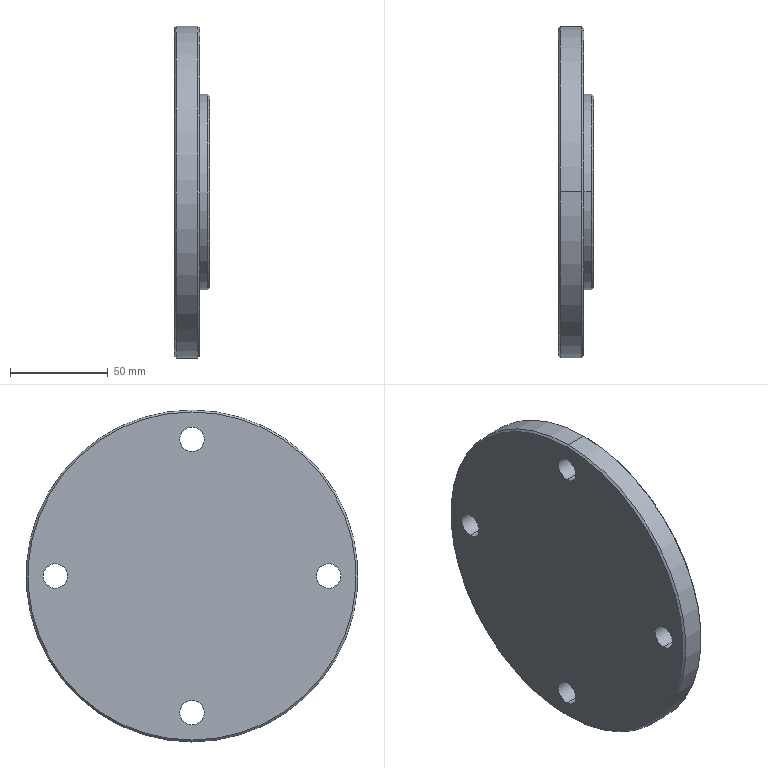Part | SolidWorks | features Chamfer 1, CirPattern 1, ICE 1, Revolution 1 | 1 solid | 26 faces | box 18 x 170 x 170 mm | volume 307921 mm3 | cylinder 14 | cone 8 | plane 4 | commonest cylinder face diameters 12.5 x8 70 x2 100 x2 170 x2
STEP:
#1=CARTESIAN_POINT('',(13.,0.,-84.));
#2=VERTEX_POINT('',#1);
#3=CARTESIAN_POINT('',(13.,0.,84.));
#4=VERTEX_POINT('',#3);
#5=CARTESIAN_POINT('',(13.,0.,0.));
#6=DIRECTION('',(1.,0.,0.));
#7=DIRECTION('',(0.,0.,1.));
#8=AXIS2_PLACEMENT_3D('',#5,#6,#7);
#9=CIRCLE('',#8,84.);
#10=EDGE_CURVE('',#2,#4,#9,.T.);
#11=ORIENTED_EDGE('',*,*,#10,.F.);
#12=CARTESIAN_POINT('',(12.,0.,-85.));
#13=VERTEX_POINT('',#12);
#14=CARTESIAN_POINT('',(12.,0.,-85.));
#15=DIRECTION('',(-0.7071,0.,-0.7071));
#16=VECTOR('',#15,1000.);
#17=LINE('',#14,#16);
#18=EDGE_CURVE('',#2,#13,#17,.T.);
#19=ORIENTED_EDGE('',*,*,#18,.T.);
#20=CARTESIAN_POINT('',(12.,0.,85.));
#21=VERTEX_POINT('',#20);
#22=CARTESIAN_POINT('',(12.,0.,0.));
#23=DIRECTION('',(-1.,0.,0.));
#24=DIRECTION('',(0.,0.,1.));
#25=AXIS2_PLACEMENT_3D('',#22,#23,#24);
#26=CIRCLE('',#25,85.);
#27=EDGE_CURVE('',#21,#13,#26,.T.);
#28=ORIENTED_EDGE('',*,*,#27,.F.);
#29=CARTESIAN_POINT('',(12.,0.,85.));
#30=DIRECTION('',(-0.7071,0.,0.7071));
#31=VECTOR('',#30,1000.);
#32=LINE('',#29,#31);
#33=EDGE_CURVE('',#4,#21,#32,.T.);
#34=ORIENTED_EDGE('',*,*,#33,.F.);
#35=EDGE_LOOP('',(#11,#19,#28,#34));
#36=FACE_OUTER_BOUND('',#35,.T.);
#37=CARTESIAN_POINT('',(12.,0.,0.));
#38=DIRECTION('',(-1.,0.,0.));
#39=DIRECTION('',(0.,0.,1.));
#40=AXIS2_PLACEMENT_3D('',#37,#38,#39);
#41=CONICAL_SURFACE('',#40,85.,0.7854);
#42=ADVANCED_FACE('',(#36),#41,.T.);
#43=CARTESIAN_POINT('',(0.,0.,84.));
#44=VERTEX_POINT('',#43);
#45=CARTESIAN_POINT('',(0.,0.,-84.));
#46=VERTEX_POINT('',#45);
#47=CARTESIAN_POINT('',(0.,0.,0.));
#48=DIRECTION('',(-1.,0.,0.));
#49=DIRECTION('',(0.,0.,-1.));
#50=AXIS2_PLACEMENT_3D('',#47,#48,#49);
#51=CIRCLE('',#50,84.);
#52=EDGE_CURVE('',#44,#46,#51,.T.);
#53=ORIENTED_EDGE('',*,*,#52,.F.);
#54=CARTESIAN_POINT('',(1.,0.,85.));
#55=VERTEX_POINT('',#54);
#56=CARTESIAN_POINT('',(0.,0.,84.));
#57=DIRECTION('',(0.7071,0.,0.7071));
#58=VECTOR('',#57,1000.);
#59=LINE('',#56,#58);
#60=EDGE_CURVE('',#44,#55,#59,.T.);
#61=ORIENTED_EDGE('',*,*,#60,.T.);
#62=CARTESIAN_POINT('',(1.,0.,-85.));
#63=VERTEX_POINT('',#62);
#64=CARTESIAN_POINT('',(1.,0.,0.));
#65=DIRECTION('',(1.,0.,0.));
#66=DIRECTION('',(0.,0.,-1.));
#67=AXIS2_PLACEMENT_3D('',#64,#65,#66);
#68=CIRCLE('',#67,85.);
#69=EDGE_CURVE('',#63,#55,#68,.T.);
#70=ORIENTED_EDGE('',*,*,#69,.F.);
#71=CARTESIAN_POINT('',(0.,0.,-84.));
#72=DIRECTION('',(0.7071,0.,-0.7071));
#73=VECTOR('',#72,1000.);
#74=LINE('',#71,#73);
#75=EDGE_CURVE('',#46,#63,#74,.T.);
#76=ORIENTED_EDGE('',*,*,#75,.F.);
#77=EDGE_LOOP('',(#53,#61,#70,#76));
#78=FACE_OUTER_BOUND('',#77,.T.);
#79=CARTESIAN_POINT('',(0.,0.,0.));
#80=DIRECTION('',(1.,0.,0.));
#81=DIRECTION('',(0.,0.,-1.));
#82=AXIS2_PLACEMENT_3D('',#79,#80,#81);
#83=CONICAL_SURFACE('',#82,84.,0.7854);
#84=ADVANCED_FACE('',(#78),#83,.T.);
#85=CARTESIAN_POINT('',(18.,0.,-49.));
#86=VERTEX_POINT('',#85);
#87=CARTESIAN_POINT('',(18.,0.,49.));
#88=VERTEX_POINT('',#87);
#89=CARTESIAN_POINT('',(18.,0.,0.));
#90=DIRECTION('',(1.,0.,0.));
#91=DIRECTION('',(0.,0.,1.));
#92=AXIS2_PLACEMENT_3D('',#89,#90,#91);
#93=CIRCLE('',#92,49.);
#94=EDGE_CURVE('',#86,#88,#93,.T.);
#95=ORIENTED_EDGE('',*,*,#94,.F.);
#96=CARTESIAN_POINT('',(17.,0.,-50.));
#97=VERTEX_POINT('',#96);
#98=CARTESIAN_POINT('',(17.,0.,-50.));
#99=DIRECTION('',(-0.7071,0.,-0.7071));
#100=VECTOR('',#99,1000.);
#101=LINE('',#98,#100);
#102=EDGE_CURVE('',#86,#97,#101,.T.);
#103=ORIENTED_EDGE('',*,*,#102,.T.);
#104=CARTESIAN_POINT('',(17.,0.,50.));
#105=VERTEX_POINT('',#104);
#106=CARTESIAN_POINT('',(17.,0.,0.));
#107=DIRECTION('',(-1.,0.,0.));
#108=DIRECTION('',(0.,0.,1.));
#109=AXIS2_PLACEMENT_3D('',#106,#107,#108);
#110=CIRCLE('',#109,50.);
#111=EDGE_CURVE('',#105,#97,#110,.T.);
#112=ORIENTED_EDGE('',*,*,#111,.F.);
#113=CARTESIAN_POINT('',(17.,0.,50.));
#114=DIRECTION('',(-0.7071,0.,0.7071));
#115=VECTOR('',#114,1000.);
#116=LINE('',#113,#115);
#117=EDGE_CURVE('',#88,#105,#116,.T.);
#118=ORIENTED_EDGE('',*,*,#117,.F.);
#119=EDGE_LOOP('',(#95,#103,#112,#118));
#120=FACE_OUTER_BOUND('',#119,.T.);
#121=CARTESIAN_POINT('',(17.,0.,0.));
#122=DIRECTION('',(-1.,0.,0.));
#123=DIRECTION('',(0.,0.,1.));
#124=AXIS2_PLACEMENT_3D('',#121,#122,#123);
#125=CONICAL_SURFACE('',#124,50.,0.7854);
#126=ADVANCED_FACE('',(#120),#125,.T.);
#127=CARTESIAN_POINT('',(17.,0.,35.));
#128=VERTEX_POINT('',#127);
#129=CARTESIAN_POINT('',(17.,0.,-35.));
#130=VERTEX_POINT('',#129);
#131=CARTESIAN_POINT('',(17.,0.,0.));
#132=DIRECTION('',(1.,0.,0.));
#133=DIRECTION('',(0.,0.,1.));
#134=AXIS2_PLACEMENT_3D('',#131,#132,#133);
#135=CIRCLE('',#134,35.);
#136=EDGE_CURVE('',#128,#130,#135,.T.);
#137=ORIENTED_EDGE('',*,*,#136,.F.);
#138=CARTESIAN_POINT('',(18.,0.,36.));
#139=VERTEX_POINT('',#138);
#140=CARTESIAN_POINT('',(18.,0.,36.));
#141=DIRECTION('',(0.7071,0.,0.7071));
#142=VECTOR('',#141,1000.);
#143=LINE('',#140,#142);
#144=EDGE_CURVE('',#128,#139,#143,.T.);
#145=ORIENTED_EDGE('',*,*,#144,.T.);
#146=CARTESIAN_POINT('',(18.,0.,-36.));
#147=VERTEX_POINT('',#146);
#148=CARTESIAN_POINT('',(18.,0.,0.));
#149=DIRECTION('',(-1.,0.,0.));
#150=DIRECTION('',(0.,0.,1.));
#151=AXIS2_PLACEMENT_3D('',#148,#149,#150);
#152=CIRCLE('',#151,36.);
#153=EDGE_CURVE('',#147,#139,#152,.T.);
#154=ORIENTED_EDGE('',*,*,#153,.F.);
#155=CARTESIAN_POINT('',(18.,0.,-36.));
#156=DIRECTION('',(0.7071,0.,-0.7071));
#157=VECTOR('',#156,1000.);
#158=LINE('',#155,#157);
#159=EDGE_CURVE('',#130,#147,#158,.T.);
#160=ORIENTED_EDGE('',*,*,#159,.F.);
#161=EDGE_LOOP('',(#137,#145,#154,#160));
#162=FACE_OUTER_BOUND('',#161,.T.);
#163=CARTESIAN_POINT('',(18.,0.,0.));
#164=DIRECTION('',(1.,0.,0.));
#165=DIRECTION('',(0.,0.,-1.));
#166=AXIS2_PLACEMENT_3D('',#163,#164,#165);
#167=CONICAL_SURFACE('',#166,36.,0.7854);
#168=ADVANCED_FACE('',(#162),#167,.F.);
#169=CARTESIAN_POINT('',(13.,-70.,-6.25));
#170=VERTEX_POINT('',#169);
#171=CARTESIAN_POINT('',(13.,-70.,6.25));
#172=VERTEX_POINT('',#171);
#173=CARTESIAN_POINT('',(13.,-70.,0.));
#174=DIRECTION('',(-1.,0.,0.));
#175=DIRECTION('',(0.,0.,1.));
#176=AXIS2_PLACEMENT_3D('',#173,#174,#175);
#177=CIRCLE('',#176,6.25);
#178=EDGE_CURVE('',#170,#172,#177,.T.);
#179=ORIENTED_EDGE('',*,*,#178,.F.);
#180=CARTESIAN_POINT('',(0.,-70.,-6.25));
#181=VERTEX_POINT('',#180);
#182=CARTESIAN_POINT('',(18.,-70.,-6.25));
#183=DIRECTION('',(-1.,0.,0.));
#184=VECTOR('',#183,1000.);
#185=LINE('',#182,#184);
#186=EDGE_CURVE('',#170,#181,#185,.T.);
#187=ORIENTED_EDGE('',*,*,#186,.T.);
#188=CARTESIAN_POINT('',(0.,-70.,6.25));
#189=VERTEX_POINT('',#188);
#190=CARTESIAN_POINT('',(0.,-70.,0.));
#191=DIRECTION('',(-1.,0.,0.));
#192=DIRECTION('',(0.,0.,-1.));
#193=AXIS2_PLACEMENT_3D('',#190,#191,#192);
#194=CIRCLE('',#193,6.25);
#195=EDGE_CURVE('',#181,#189,#194,.T.);
#196=ORIENTED_EDGE('',*,*,#195,.T.);
#197=CARTESIAN_POINT('',(18.,-70.,6.25));
#198=DIRECTION('',(-1.,0.,0.));
#199=VECTOR('',#198,1000.);
#200=LINE('',#197,#199);
#201=EDGE_CURVE('',#172,#189,#200,.T.);
#202=ORIENTED_EDGE('',*,*,#201,.F.);
#203=EDGE_LOOP('',(#179,#187,#196,#202));
#204=FACE_OUTER_BOUND('',#203,.T.);
#205=CARTESIAN_POINT('',(18.,-70.,0.));
#206=DIRECTION('',(-1.,0.,0.));
#207=DIRECTION('',(0.,0.,1.));
#208=AXIS2_PLACEMENT_3D('',#205,#206,#207);
#209=CYLINDRICAL_SURFACE('',#208,6.25);
#210=ADVANCED_FACE('',(#204),#209,.F.);
#211=CARTESIAN_POINT('',(13.,0.,63.75));
#212=VERTEX_POINT('',#211);
#213=CARTESIAN_POINT('',(13.,0.,76.25));
#214=VERTEX_POINT('',#213);
#215=CARTESIAN_POINT('',(13.,0.,70.));
#216=DIRECTION('',(-1.,0.,0.));
#217=DIRECTION('',(0.,0.,1.));
#218=AXIS2_PLACEMENT_3D('',#215,#216,#217);
#219=CIRCLE('',#218,6.25);
#220=EDGE_CURVE('',#212,#214,#219,.T.);
#221=ORIENTED_EDGE('',*,*,#220,.F.);
#222=CARTESIAN_POINT('',(0.,0.,63.75));
#223=VERTEX_POINT('',#222);
#224=CARTESIAN_POINT('',(18.,0.,63.75));
#225=DIRECTION('',(-1.,0.,0.));
#226=VECTOR('',#225,1000.);
#227=LINE('',#224,#226);
#228=EDGE_CURVE('',#212,#223,#227,.T.);
#229=ORIENTED_EDGE('',*,*,#228,.T.);
#230=CARTESIAN_POINT('',(0.,0.,76.25));
#231=VERTEX_POINT('',#230);
#232=CARTESIAN_POINT('',(0.,0.,70.));
#233=DIRECTION('',(-1.,0.,0.));
#234=DIRECTION('',(0.,-1.,0.));
#235=AXIS2_PLACEMENT_3D('',#232,#233,#234);
#236=CIRCLE('',#235,6.25);
#237=EDGE_CURVE('',#223,#231,#236,.T.);
#238=ORIENTED_EDGE('',*,*,#237,.T.);
#239=CARTESIAN_POINT('',(18.,0.,76.25));
#240=DIRECTION('',(-1.,0.,0.));
#241=VECTOR('',#240,1000.);
#242=LINE('',#239,#241);
#243=EDGE_CURVE('',#214,#231,#242,.T.);
#244=ORIENTED_EDGE('',*,*,#243,.F.);
#245=EDGE_LOOP('',(#221,#229,#238,#244));
#246=FACE_OUTER_BOUND('',#245,.T.);
#247=CARTESIAN_POINT('',(18.,0.,70.));
#248=DIRECTION('',(-1.,0.,0.));
#249=DIRECTION('',(0.,0.,1.));
#250=AXIS2_PLACEMENT_3D('',#247,#248,#249);
#251=CYLINDRICAL_SURFACE('',#250,6.25);
#252=ADVANCED_FACE('',(#246),#251,.F.);
#253=CARTESIAN_POINT('',(13.,0.,-76.25));
#254=VERTEX_POINT('',#253);
#255=CARTESIAN_POINT('',(13.,0.,-63.75));
#256=VERTEX_POINT('',#255);
#257=CARTESIAN_POINT('',(13.,0.,-70.));
#258=DIRECTION('',(-1.,0.,0.));
#259=DIRECTION('',(0.,0.,1.));
#260=AXIS2_PLACEMENT_3D('',#257,#258,#259);
#261=CIRCLE('',#260,6.25);
#262=EDGE_CURVE('',#254,#256,#261,.T.);
#263=ORIENTED_EDGE('',*,*,#262,.F.);
#264=CARTESIAN_POINT('',(0.,0.,-76.25));
#265=VERTEX_POINT('',#264);
#266=CARTESIAN_POINT('',(18.,0.,-76.25));
#267=DIRECTION('',(-1.,0.,0.));
#268=VECTOR('',#267,1000.);
#269=LINE('',#266,#268);
#270=EDGE_CURVE('',#254,#265,#269,.T.);
#271=ORIENTED_EDGE('',*,*,#270,.T.);
#272=CARTESIAN_POINT('',(0.,0.,-63.75));
#273=VERTEX_POINT('',#272);
#274=CARTESIAN_POINT('',(0.,0.,-70.));
#275=DIRECTION('',(-1.,0.,0.));
#276=DIRECTION('',(0.,1.,0.));
#277=AXIS2_PLACEMENT_3D('',#274,#275,#276);
#278=CIRCLE('',#277,6.25);
#279=EDGE_CURVE('',#265,#273,#278,.T.);
#280=ORIENTED_EDGE('',*,*,#279,.T.);
#281=CARTESIAN_POINT('',(18.,0.,-63.75));
#282=DIRECTION('',(-1.,0.,0.));
#283=VECTOR('',#282,1000.);
#284=LINE('',#281,#283);
#285=EDGE_CURVE('',#256,#273,#284,.T.);
#286=ORIENTED_EDGE('',*,*,#285,.F.);
#287=EDGE_LOOP('',(#263,#271,#280,#286));
#288=FACE_OUTER_BOUND('',#287,.T.);
#289=CARTESIAN_POINT('',(18.,0.,-70.));
#290=DIRECTION('',(-1.,0.,0.));
#291=DIRECTION('',(0.,0.,1.));
#292=AXIS2_PLACEMENT_3D('',#289,#290,#291);
#293=CYLINDRICAL_SURFACE('',#292,6.25);
#294=ADVANCED_FACE('',(#288),#293,.F.);
#295=CARTESIAN_POINT('',(13.,70.,-6.25));
#296=VERTEX_POINT('',#295);
#297=CARTESIAN_POINT('',(13.,70.,6.25));
#298=VERTEX_POINT('',#297);
#299=CARTESIAN_POINT('',(13.,70.,0.));
#300=DIRECTION('',(-1.,0.,0.));
#301=DIRECTION('',(0.,0.,1.));
#302=AXIS2_PLACEMENT_3D('',#299,#300,#301);
#303=CIRCLE('',#302,6.25);
#304=EDGE_CURVE('',#296,#298,#303,.T.);
#305=ORIENTED_EDGE('',*,*,#304,.F.);
#306=CARTESIAN_POINT('',(0.,70.,-6.25));
#307=VERTEX_POINT('',#306);
#308=CARTESIAN_POINT('',(18.,70.,-6.25));
#309=DIRECTION('',(-1.,0.,0.));
#310=VECTOR('',#309,1000.);
#311=LINE('',#308,#310);
#312=EDGE_CURVE('',#296,#307,#311,.T.);
#313=ORIENTED_EDGE('',*,*,#312,.T.);
#314=CARTESIAN_POINT('',(0.,70.,6.25));
#315=VERTEX_POINT('',#314);
#316=CARTESIAN_POINT('',(0.,70.,0.));
#317=DIRECTION('',(-1.,0.,0.));
#318=DIRECTION('',(0.,0.,1.));
#319=AXIS2_PLACEMENT_3D('',#316,#317,#318);
#320=CIRCLE('',#319,6.25);
#321=EDGE_CURVE('',#307,#315,#320,.T.);
#322=ORIENTED_EDGE('',*,*,#321,.T.);
#323=CARTESIAN_POINT('',(18.,70.,6.25));
#324=DIRECTION('',(-1.,0.,0.));
#325=VECTOR('',#324,1000.);
#326=LINE('',#323,#325);
#327=EDGE_CURVE('',#298,#315,#326,.T.);
#328=ORIENTED_EDGE('',*,*,#327,.F.);
#329=EDGE_LOOP('',(#305,#313,#322,#328));
#330=FACE_OUTER_BOUND('',#329,.T.);
#331=CARTESIAN_POINT('',(18.,70.,0.));
#332=DIRECTION('',(-1.,0.,0.));
#333=DIRECTION('',(0.,0.,1.));
#334=AXIS2_PLACEMENT_3D('',#331,#332,#333);
#335=CYLINDRICAL_SURFACE('',#334,6.25);
#336=ADVANCED_FACE('',(#330),#335,.F.);
#337=ORIENTED_EDGE('',*,*,#136,.T.);
#338=CARTESIAN_POINT('',(13.,0.,-35.));
#339=VERTEX_POINT('',#338);
#340=CARTESIAN_POINT('',(0.,0.,-35.));
#341=DIRECTION('',(-1.,0.,0.));
#342=VECTOR('',#341,1000.);
#343=LINE('',#340,#342);
#344=EDGE_CURVE('',#130,#339,#343,.T.);
#345=ORIENTED_EDGE('',*,*,#344,.T.);
#346=CARTESIAN_POINT('',(13.,0.,35.));
#347=VERTEX_POINT('',#346);
#348=CARTESIAN_POINT('',(13.,0.,0.));
#349=DIRECTION('',(-1.,0.,0.));
#350=DIRECTION('',(0.,0.,1.));
#351=AXIS2_PLACEMENT_3D('',#348,#349,#350);
#352=CIRCLE('',#351,35.);
#353=EDGE_CURVE('',#339,#347,#352,.T.);
#354=ORIENTED_EDGE('',*,*,#353,.T.);
#355=CARTESIAN_POINT('',(0.,0.,35.));
#356=DIRECTION('',(-1.,0.,0.));
#357=VECTOR('',#356,1000.);
#358=LINE('',#355,#357);
#359=EDGE_CURVE('',#128,#347,#358,.T.);
#360=ORIENTED_EDGE('',*,*,#359,.F.);
#361=EDGE_LOOP('',(#337,#345,#354,#360));
#362=FACE_OUTER_BOUND('',#361,.T.);
#363=CARTESIAN_POINT('',(0.,0.,0.));
#364=DIRECTION('',(-1.,0.,0.));
#365=DIRECTION('',(0.,0.,1.));
#366=AXIS2_PLACEMENT_3D('',#363,#364,#365);
#367=CYLINDRICAL_SURFACE('',#366,35.);
#368=ADVANCED_FACE('',(#362),#367,.F.);
#369=ORIENTED_EDGE('',*,*,#111,.T.);
#370=CARTESIAN_POINT('',(13.,0.,-50.));
#371=VERTEX_POINT('',#370);
#372=CARTESIAN_POINT('',(0.,0.,-50.));
#373=DIRECTION('',(-1.,0.,0.));
#374=VECTOR('',#373,1000.);
#375=LINE('',#372,#374);
#376=EDGE_CURVE('',#97,#371,#375,.T.);
#377=ORIENTED_EDGE('',*,*,#376,.T.);
#378=CARTESIAN_POINT('',(13.,0.,50.));
#379=VERTEX_POINT('',#378);
#380=CARTESIAN_POINT('',(13.,0.,0.));
#381=DIRECTION('',(-1.,0.,0.));
#382=DIRECTION('',(0.,0.,1.));
#383=AXIS2_PLACEMENT_3D('',#380,#381,#382);
#384=CIRCLE('',#383,50.);
#385=EDGE_CURVE('',#379,#371,#384,.T.);
#386=ORIENTED_EDGE('',*,*,#385,.F.);
#387=CARTESIAN_POINT('',(0.,0.,50.));
#388=DIRECTION('',(-1.,0.,0.));
#389=VECTOR('',#388,1000.);
#390=LINE('',#387,#389);
#391=EDGE_CURVE('',#105,#379,#390,.T.);
#392=ORIENTED_EDGE('',*,*,#391,.F.);
#393=EDGE_LOOP('',(#369,#377,#386,#392));
#394=FACE_OUTER_BOUND('',#393,.T.);
#395=CARTESIAN_POINT('',(0.,0.,0.));
#396=DIRECTION('',(-1.,0.,0.));
#397=DIRECTION('',(0.,0.,1.));
#398=AXIS2_PLACEMENT_3D('',#395,#396,#397);
#399=CYLINDRICAL_SURFACE('',#398,50.);
#400=ADVANCED_FACE('',(#394),#399,.T.);
#401=ORIENTED_EDGE('',*,*,#27,.T.);
#402=CARTESIAN_POINT('',(0.,0.,-85.));
#403=DIRECTION('',(-1.,0.,0.));
#404=VECTOR('',#403,1000.);
#405=LINE('',#402,#404);
#406=EDGE_CURVE('',#13,#63,#405,.T.);
#407=ORIENTED_EDGE('',*,*,#406,.T.);
#408=ORIENTED_EDGE('',*,*,#69,.T.);
#409=CARTESIAN_POINT('',(0.,0.,85.));
#410=DIRECTION('',(-1.,0.,0.));
#411=VECTOR('',#410,1000.);
#412=LINE('',#409,#411);
#413=EDGE_CURVE('',#21,#55,#412,.T.);
#414=ORIENTED_EDGE('',*,*,#413,.F.);
#415=EDGE_LOOP('',(#401,#407,#408,#414));
#416=FACE_OUTER_BOUND('',#415,.T.);
#417=CARTESIAN_POINT('',(0.,0.,0.));
#418=DIRECTION('',(-1.,0.,0.));
#419=DIRECTION('',(0.,0.,1.));
#420=AXIS2_PLACEMENT_3D('',#417,#418,#419);
#421=CYLINDRICAL_SURFACE('',#420,85.);
#422=ADVANCED_FACE('',(#416),#421,.T.);
#423=CARTESIAN_POINT('',(0.,0.,0.));
#424=DIRECTION('',(-1.,0.,0.));
#425=DIRECTION('',(0.,0.,-1.));
#426=AXIS2_PLACEMENT_3D('',#423,#424,#425);
#427=CIRCLE('',#426,84.);
#428=EDGE_CURVE('',#46,#44,#427,.T.);
#429=ORIENTED_EDGE('',*,*,#428,.T.);
#430=ORIENTED_EDGE('',*,*,#52,.T.);
#431=EDGE_LOOP('',(#429,#430));
#432=FACE_OUTER_BOUND('',#431,.T.);
#433=CARTESIAN_POINT('',(0.,-70.,0.));
#434=DIRECTION('',(-1.,0.,0.));
#435=DIRECTION('',(0.,0.,-1.));
#436=AXIS2_PLACEMENT_3D('',#433,#434,#435);
#437=CIRCLE('',#436,6.25);
#438=EDGE_CURVE('',#189,#181,#437,.T.);
#439=ORIENTED_EDGE('',*,*,#438,.F.);
#440=ORIENTED_EDGE('',*,*,#195,.F.);
#441=EDGE_LOOP('',(#439,#440));
#442=FACE_BOUND('',#441,.T.);
#443=CARTESIAN_POINT('',(0.,0.,70.));
#444=DIRECTION('',(-1.,0.,0.));
#445=DIRECTION('',(0.,-1.,0.));
#446=AXIS2_PLACEMENT_3D('',#443,#444,#445);
#447=CIRCLE('',#446,6.25);
#448=EDGE_CURVE('',#231,#223,#447,.T.);
#449=ORIENTED_EDGE('',*,*,#448,.F.);
#450=ORIENTED_EDGE('',*,*,#237,.F.);
#451=EDGE_LOOP('',(#449,#450));
#452=FACE_BOUND('',#451,.T.);
#453=CARTESIAN_POINT('',(0.,0.,-70.));
#454=DIRECTION('',(-1.,0.,0.));
#455=DIRECTION('',(0.,1.,0.));
#456=AXIS2_PLACEMENT_3D('',#453,#454,#455);
#457=CIRCLE('',#456,6.25);
#458=EDGE_CURVE('',#273,#265,#457,.T.);
#459=ORIENTED_EDGE('',*,*,#458,.F.);
#460=ORIENTED_EDGE('',*,*,#279,.F.);
#461=EDGE_LOOP('',(#459,#460));
#462=FACE_BOUND('',#461,.T.);
#463=CARTESIAN_POINT('',(0.,70.,0.));
#464=DIRECTION('',(-1.,0.,0.));
#465=DIRECTION('',(0.,0.,1.));
#466=AXIS2_PLACEMENT_3D('',#463,#464,#465);
#467=CIRCLE('',#466,6.25);
#468=EDGE_CURVE('',#315,#307,#467,.T.);
#469=ORIENTED_EDGE('',*,*,#468,.F.);
#470=ORIENTED_EDGE('',*,*,#321,.F.);
#471=EDGE_LOOP('',(#469,#470));
#472=FACE_BOUND('',#471,.T.);
#473=CARTESIAN_POINT('',(0.,0.,0.));
#474=DIRECTION('',(1.,0.,0.));
#475=DIRECTION('',(0.,0.,-1.));
#476=AXIS2_PLACEMENT_3D('',#473,#474,#475);
#477=PLANE('',#476);
#478=ADVANCED_FACE('',(#432,#442,#452,#462,#472),#477,.F.);
#479=ORIENTED_EDGE('',*,*,#406,.F.);
#480=CARTESIAN_POINT('',(12.,0.,0.));
#481=DIRECTION('',(-1.,0.,0.));
#482=DIRECTION('',(0.,0.,1.));
#483=AXIS2_PLACEMENT_3D('',#480,#481,#482);
#484=CIRCLE('',#483,85.);
#485=EDGE_CURVE('',#13,#21,#484,.T.);
#486=ORIENTED_EDGE('',*,*,#485,.T.);
#487=ORIENTED_EDGE('',*,*,#413,.T.);
#488=CARTESIAN_POINT('',(1.,0.,0.));
#489=DIRECTION('',(1.,0.,0.));
#490=DIRECTION('',(0.,0.,-1.));
#491=AXIS2_PLACEMENT_3D('',#488,#489,#490);
#492=CIRCLE('',#491,85.);
#493=EDGE_CURVE('',#55,#63,#492,.T.);
#494=ORIENTED_EDGE('',*,*,#493,.T.);
#495=EDGE_LOOP('',(#479,#486,#487,#494));
#496=FACE_OUTER_BOUND('',#495,.T.);
#497=CARTESIAN_POINT('',(0.,0.,0.));
#498=DIRECTION('',(-1.,0.,0.));
#499=DIRECTION('',(0.,0.,1.));
#500=AXIS2_PLACEMENT_3D('',#497,#498,#499);
#501=CYLINDRICAL_SURFACE('',#500,85.);
#502=ADVANCED_FACE('',(#496),#501,.T.);
#503=CARTESIAN_POINT('',(13.,0.,0.));
#504=DIRECTION('',(1.,0.,0.));
#505=DIRECTION('',(0.,0.,1.));
#506=AXIS2_PLACEMENT_3D('',#503,#504,#505);
#507=CIRCLE('',#506,84.);
#508=EDGE_CURVE('',#4,#2,#507,.T.);
#509=ORIENTED_EDGE('',*,*,#508,.T.);
#510=ORIENTED_EDGE('',*,*,#10,.T.);
#511=EDGE_LOOP('',(#509,#510));
#512=FACE_OUTER_BOUND('',#511,.T.);
#513=CARTESIAN_POINT('',(13.,-70.,0.));
#514=DIRECTION('',(-1.,0.,0.));
#515=DIRECTION('',(0.,0.,1.));
#516=AXIS2_PLACEMENT_3D('',#513,#514,#515);
#517=CIRCLE('',#516,6.25);
#518=EDGE_CURVE('',#172,#170,#517,.T.);
#519=ORIENTED_EDGE('',*,*,#518,.T.);
#520=ORIENTED_EDGE('',*,*,#178,.T.);
#521=EDGE_LOOP('',(#519,#520));
#522=FACE_BOUND('',#521,.T.);
#523=CARTESIAN_POINT('',(13.,0.,70.));
#524=DIRECTION('',(-1.,0.,0.));
#525=DIRECTION('',(0.,0.,1.));
#526=AXIS2_PLACEMENT_3D('',#523,#524,#525);
#527=CIRCLE('',#526,6.25);
#528=EDGE_CURVE('',#214,#212,#527,.T.);
#529=ORIENTED_EDGE('',*,*,#528,.T.);
#530=ORIENTED_EDGE('',*,*,#220,.T.);
#531=EDGE_LOOP('',(#529,#530));
#532=FACE_BOUND('',#531,.T.);
#533=CARTESIAN_POINT('',(13.,0.,-70.));
#534=DIRECTION('',(-1.,0.,0.));
#535=DIRECTION('',(0.,0.,1.));
#536=AXIS2_PLACEMENT_3D('',#533,#534,#535);
#537=CIRCLE('',#536,6.25);
#538=EDGE_CURVE('',#256,#254,#537,.T.);
#539=ORIENTED_EDGE('',*,*,#538,.T.);
#540=ORIENTED_EDGE('',*,*,#262,.T.);
#541=EDGE_LOOP('',(#539,#540));
#542=FACE_BOUND('',#541,.T.);
#543=CARTESIAN_POINT('',(13.,70.,0.));
#544=DIRECTION('',(-1.,0.,0.));
#545=DIRECTION('',(0.,0.,1.));
#546=AXIS2_PLACEMENT_3D('',#543,#544,#545);
#547=CIRCLE('',#546,6.25);
#548=EDGE_CURVE('',#298,#296,#547,.T.);
#549=ORIENTED_EDGE('',*,*,#548,.T.);
#550=ORIENTED_EDGE('',*,*,#304,.T.);
#551=EDGE_LOOP('',(#549,#550));
#552=FACE_BOUND('',#551,.T.);
#553=ORIENTED_EDGE('',*,*,#385,.T.);
#554=CARTESIAN_POINT('',(13.,0.,0.));
#555=DIRECTION('',(-1.,0.,0.));
#556=DIRECTION('',(0.,0.,1.));
#557=AXIS2_PLACEMENT_3D('',#554,#555,#556);
#558=CIRCLE('',#557,50.);
#559=EDGE_CURVE('',#371,#379,#558,.T.);
#560=ORIENTED_EDGE('',*,*,#559,.T.);
#561=EDGE_LOOP('',(#553,#560));
#562=FACE_BOUND('',#561,.T.);
#563=CARTESIAN_POINT('',(13.,85.,0.));
#564=DIRECTION('',(-1.,0.,0.));
#565=DIRECTION('',(0.,0.,1.));
#566=AXIS2_PLACEMENT_3D('',#563,#564,#565);
#567=PLANE('',#566);
#568=ADVANCED_FACE('',(#512,#522,#532,#542,#552,#562),#567,.F.);
#569=ORIENTED_EDGE('',*,*,#376,.F.);
#570=CARTESIAN_POINT('',(17.,0.,0.));
#571=DIRECTION('',(-1.,0.,0.));
#572=DIRECTION('',(0.,0.,1.));
#573=AXIS2_PLACEMENT_3D('',#570,#571,#572);
#574=CIRCLE('',#573,50.);
#575=EDGE_CURVE('',#97,#105,#574,.T.);
#576=ORIENTED_EDGE('',*,*,#575,.T.);
#577=ORIENTED_EDGE('',*,*,#391,.T.);
#578=ORIENTED_EDGE('',*,*,#559,.F.);
#579=EDGE_LOOP('',(#569,#576,#577,#578));
#580=FACE_OUTER_BOUND('',#579,.T.);
#581=CARTESIAN_POINT('',(0.,0.,0.));
#582=DIRECTION('',(-1.,0.,0.));
#583=DIRECTION('',(0.,0.,1.));
#584=AXIS2_PLACEMENT_3D('',#581,#582,#583);
#585=CYLINDRICAL_SURFACE('',#584,50.);
#586=ADVANCED_FACE('',(#580),#585,.T.);
#587=ORIENTED_EDGE('',*,*,#153,.T.);
#588=CARTESIAN_POINT('',(18.,0.,0.));
#589=DIRECTION('',(-1.,0.,0.));
#590=DIRECTION('',(0.,0.,1.));
#591=AXIS2_PLACEMENT_3D('',#588,#589,#590);
#592=CIRCLE('',#591,36.);
#593=EDGE_CURVE('',#139,#147,#592,.T.);
#594=ORIENTED_EDGE('',*,*,#593,.T.);
#595=EDGE_LOOP('',(#587,#594));
#596=FACE_BOUND('',#595,.T.);
#597=CARTESIAN_POINT('',(18.,0.,0.));
#598=DIRECTION('',(1.,0.,0.));
#599=DIRECTION('',(0.,0.,1.));
#600=AXIS2_PLACEMENT_3D('',#597,#598,#599);
#601=CIRCLE('',#600,49.);
#602=EDGE_CURVE('',#88,#86,#601,.T.);
#603=ORIENTED_EDGE('',*,*,#602,.T.);
#604=ORIENTED_EDGE('',*,*,#94,.T.);
#605=EDGE_LOOP('',(#603,#604));
#606=FACE_OUTER_BOUND('',#605,.T.);
#607=CARTESIAN_POINT('',(18.,50.,0.));
#608=DIRECTION('',(-1.,0.,0.));
#609=DIRECTION('',(0.,0.,1.));
#610=AXIS2_PLACEMENT_3D('',#607,#608,#609);
#611=PLANE('',#610);
#612=ADVANCED_FACE('',(#596,#606),#611,.F.);
#613=ORIENTED_EDGE('',*,*,#344,.F.);
#614=CARTESIAN_POINT('',(17.,0.,0.));
#615=DIRECTION('',(1.,0.,0.));
#616=DIRECTION('',(0.,0.,1.));
#617=AXIS2_PLACEMENT_3D('',#614,#615,#616);
#618=CIRCLE('',#617,35.);
#619=EDGE_CURVE('',#130,#128,#618,.T.);
#620=ORIENTED_EDGE('',*,*,#619,.T.);
#621=ORIENTED_EDGE('',*,*,#359,.T.);
#622=CARTESIAN_POINT('',(13.,0.,0.));
#623=DIRECTION('',(-1.,0.,0.));
#624=DIRECTION('',(0.,0.,1.));
#625=AXIS2_PLACEMENT_3D('',#622,#623,#624);
#626=CIRCLE('',#625,35.);
#627=EDGE_CURVE('',#347,#339,#626,.T.);
#628=ORIENTED_EDGE('',*,*,#627,.T.);
#629=EDGE_LOOP('',(#613,#620,#621,#628));
#630=FACE_OUTER_BOUND('',#629,.T.);
#631=CARTESIAN_POINT('',(0.,0.,0.));
#632=DIRECTION('',(-1.,0.,0.));
#633=DIRECTION('',(0.,0.,1.));
#634=AXIS2_PLACEMENT_3D('',#631,#632,#633);
#635=CYLINDRICAL_SURFACE('',#634,35.);
#636=ADVANCED_FACE('',(#630),#635,.F.);
#637=ORIENTED_EDGE('',*,*,#627,.F.);
#638=ORIENTED_EDGE('',*,*,#353,.F.);
#639=EDGE_LOOP('',(#637,#638));
#640=FACE_OUTER_BOUND('',#639,.T.);
#641=CARTESIAN_POINT('',(13.,35.,0.));
#642=DIRECTION('',(-1.,0.,0.));
#643=DIRECTION('',(0.,0.,1.));
#644=AXIS2_PLACEMENT_3D('',#641,#642,#643);
#645=PLANE('',#644);
#646=ADVANCED_FACE('',(#640),#645,.F.);
#647=ORIENTED_EDGE('',*,*,#312,.F.);
#648=ORIENTED_EDGE('',*,*,#548,.F.);
#649=ORIENTED_EDGE('',*,*,#327,.T.);
#650=ORIENTED_EDGE('',*,*,#468,.T.);
#651=EDGE_LOOP('',(#647,#648,#649,#650));
#652=FACE_OUTER_BOUND('',#651,.T.);
#653=CARTESIAN_POINT('',(18.,70.,0.));
#654=DIRECTION('',(-1.,0.,0.));
#655=DIRECTION('',(0.,0.,1.));
#656=AXIS2_PLACEMENT_3D('',#653,#654,#655);
#657=CYLINDRICAL_SURFACE('',#656,6.25);
#658=ADVANCED_FACE('',(#652),#657,.F.);
#659=ORIENTED_EDGE('',*,*,#270,.F.);
#660=ORIENTED_EDGE('',*,*,#538,.F.);
#661=ORIENTED_EDGE('',*,*,#285,.T.);
#662=ORIENTED_EDGE('',*,*,#458,.T.);
#663=EDGE_LOOP('',(#659,#660,#661,#662));
#664=FACE_OUTER_BOUND('',#663,.T.);
#665=CARTESIAN_POINT('',(18.,0.,-70.));
#666=DIRECTION('',(-1.,0.,0.));
#667=DIRECTION('',(0.,0.,1.));
#668=AXIS2_PLACEMENT_3D('',#665,#666,#667);
#669=CYLINDRICAL_SURFACE('',#668,6.25);
#670=ADVANCED_FACE('',(#664),#669,.F.);
#671=ORIENTED_EDGE('',*,*,#228,.F.);
#672=ORIENTED_EDGE('',*,*,#528,.F.);
#673=ORIENTED_EDGE('',*,*,#243,.T.);
#674=ORIENTED_EDGE('',*,*,#448,.T.);
#675=EDGE_LOOP('',(#671,#672,#673,#674));
#676=FACE_OUTER_BOUND('',#675,.T.);
#677=CARTESIAN_POINT('',(18.,0.,70.));
#678=DIRECTION('',(-1.,0.,0.));
#679=DIRECTION('',(0.,0.,1.));
#680=AXIS2_PLACEMENT_3D('',#677,#678,#679);
#681=CYLINDRICAL_SURFACE('',#680,6.25);
#682=ADVANCED_FACE('',(#676),#681,.F.);
#683=ORIENTED_EDGE('',*,*,#186,.F.);
#684=ORIENTED_EDGE('',*,*,#518,.F.);
#685=ORIENTED_EDGE('',*,*,#201,.T.);
#686=ORIENTED_EDGE('',*,*,#438,.T.);
#687=EDGE_LOOP('',(#683,#684,#685,#686));
#688=FACE_OUTER_BOUND('',#687,.T.);
#689=CARTESIAN_POINT('',(18.,-70.,0.));
#690=DIRECTION('',(-1.,0.,0.));
#691=DIRECTION('',(0.,0.,1.));
#692=AXIS2_PLACEMENT_3D('',#689,#690,#691);
#693=CYLINDRICAL_SURFACE('',#692,6.25);
#694=ADVANCED_FACE('',(#688),#693,.F.);
#695=ORIENTED_EDGE('',*,*,#144,.F.);
#696=ORIENTED_EDGE('',*,*,#619,.F.);
#697=ORIENTED_EDGE('',*,*,#159,.T.);
#698=ORIENTED_EDGE('',*,*,#593,.F.);
#699=EDGE_LOOP('',(#695,#696,#697,#698));
#700=FACE_OUTER_BOUND('',#699,.T.);
#701=CARTESIAN_POINT('',(18.,0.,0.));
#702=DIRECTION('',(1.,0.,0.));
#703=DIRECTION('',(0.,0.,-1.));
#704=AXIS2_PLACEMENT_3D('',#701,#702,#703);
#705=CONICAL_SURFACE('',#704,36.,0.7854);
#706=ADVANCED_FACE('',(#700),#705,.F.);
#707=ORIENTED_EDGE('',*,*,#102,.F.);
#708=ORIENTED_EDGE('',*,*,#602,.F.);
#709=ORIENTED_EDGE('',*,*,#117,.T.);
#710=ORIENTED_EDGE('',*,*,#575,.F.);
#711=EDGE_LOOP('',(#707,#708,#709,#710));
#712=FACE_OUTER_BOUND('',#711,.T.);
#713=CARTESIAN_POINT('',(17.,0.,0.));
#714=DIRECTION('',(-1.,0.,0.));
#715=DIRECTION('',(0.,0.,1.));
#716=AXIS2_PLACEMENT_3D('',#713,#714,#715);
#717=CONICAL_SURFACE('',#716,50.,0.7854);
#718=ADVANCED_FACE('',(#712),#717,.T.);
#719=ORIENTED_EDGE('',*,*,#60,.F.);
#720=ORIENTED_EDGE('',*,*,#428,.F.);
#721=ORIENTED_EDGE('',*,*,#75,.T.);
#722=ORIENTED_EDGE('',*,*,#493,.F.);
#723=EDGE_LOOP('',(#719,#720,#721,#722));
#724=FACE_OUTER_BOUND('',#723,.T.);
#725=CARTESIAN_POINT('',(0.,0.,0.));
#726=DIRECTION('',(1.,0.,0.));
#727=DIRECTION('',(0.,0.,-1.));
#728=AXIS2_PLACEMENT_3D('',#725,#726,#727);
#729=CONICAL_SURFACE('',#728,84.,0.7854);
#730=ADVANCED_FACE('',(#724),#729,.T.);
#731=ORIENTED_EDGE('',*,*,#18,.F.);
#732=ORIENTED_EDGE('',*,*,#508,.F.);
#733=ORIENTED_EDGE('',*,*,#33,.T.);
#734=ORIENTED_EDGE('',*,*,#485,.F.);
#735=EDGE_LOOP('',(#731,#732,#733,#734));
#736=FACE_OUTER_BOUND('',#735,.T.);
#737=CARTESIAN_POINT('',(12.,0.,0.));
#738=DIRECTION('',(-1.,0.,0.));
#739=DIRECTION('',(0.,0.,1.));
#740=AXIS2_PLACEMENT_3D('',#737,#738,#739);
#741=CONICAL_SURFACE('',#740,85.,0.7854);
#742=ADVANCED_FACE('',(#736),#741,.T.);
#743=CLOSED_SHELL('',(#42,#84,#126,#168,#210,#252,#294,#336,#368,#400,#422,#478,#502,#568,#586,#612,#636,#646,#658,#670,#682,#694,#706,#718,#730,#742));
#744=MANIFOLD_SOLID_BREP('',#743);
#745=CARTESIAN_POINT('',(0.,0.,0.));
#746=DIRECTION('',(0.,0.,1.));
#747=DIRECTION('',(1.,0.,0.));
#748=AXIS2_PLACEMENT_3D('',#745,#746,#747);
#749=(LENGTH_UNIT()NAMED_UNIT(*)SI_UNIT(.MILLI.,.METRE.));
#750=UNCERTAINTY_MEASURE_WITH_UNIT(LENGTH_MEASURE(0.00001),#749,'','');
#751=(NAMED_UNIT(*)PLANE_ANGLE_UNIT()SI_UNIT($,.RADIAN.));
#752=(NAMED_UNIT(*)SI_UNIT($,.STERADIAN.)SOLID_ANGLE_UNIT());
#753=(GEOMETRIC_REPRESENTATION_CONTEXT(3)GLOBAL_UNCERTAINTY_ASSIGNED_CONTEXT((#750))GLOBAL_UNIT_ASSIGNED_CONTEXT((#749,#751,#752))REPRESENTATION_CONTEXT('',''));
#754=ADVANCED_BREP_SHAPE_REPRESENTATION('',(#744,#748),#753);